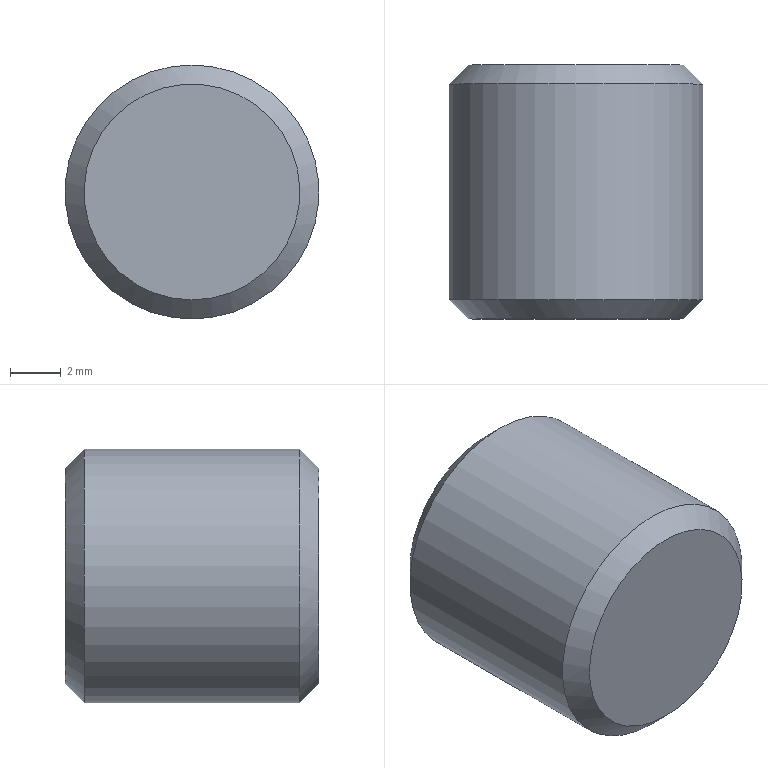Part | STEP file | WTM10.00 | 1 solid | 12 faces | box 10 x 10 x 10 mm | volume 660.357 mm3 | plane 9 | cone 2 | cylinder 1 | commonest cylinder face diameters 10 x1